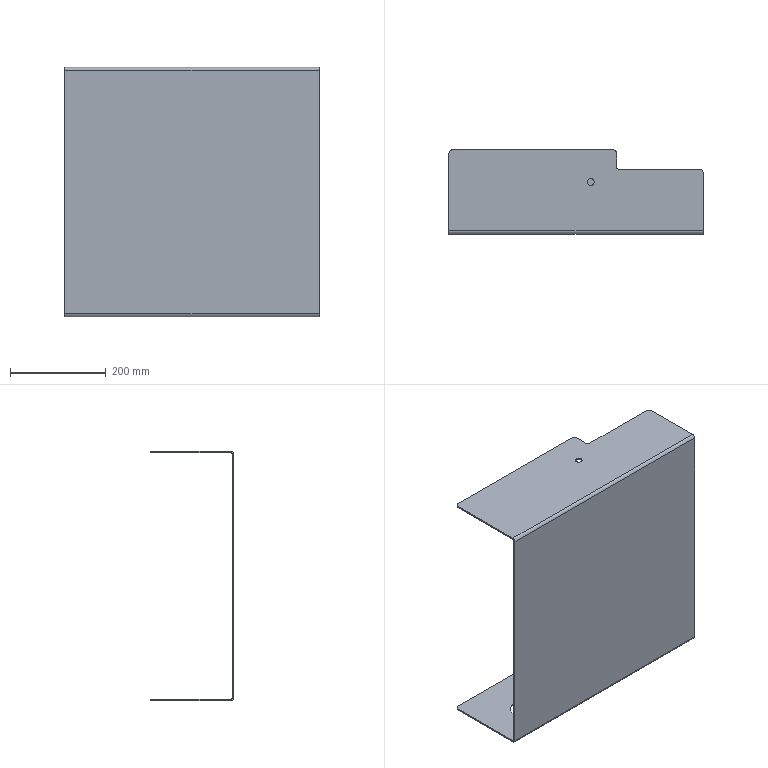Part | SolidWorks | features Fillet 2, ICE 2, FlatPattern 1, SMBaseFlange 1, SheetMetal 1 | 1 solid | 40 faces | box 530 x 175 x 520 mm | volume 1293540 mm3 | plane 22 | cylinder 18 | commonest cylinder face diameters 16 x6 6 x4 12 x2 14 x2 53 x2 100 x2
STEP:
#1=CARTESIAN_POINT('',(289.,-67.,-3.));
#2=VERTEX_POINT('',#1);
#3=CARTESIAN_POINT('',(303.,-67.,-3.));
#4=VERTEX_POINT('',#3);
#5=CARTESIAN_POINT('',(296.,-67.,-3.));
#6=DIRECTION('',(0.,0.,1.));
#7=DIRECTION('',(0.,1.,0.));
#8=AXIS2_PLACEMENT_3D('',#5,#6,#7);
#9=CIRCLE('',#8,7.);
#10=EDGE_CURVE('',#2,#4,#9,.T.);
#11=ORIENTED_EDGE('',*,*,#10,.F.);
#12=CARTESIAN_POINT('',(289.,-67.,0.));
#13=VERTEX_POINT('',#12);
#14=CARTESIAN_POINT('',(289.,-67.,-520.001));
#15=DIRECTION('',(0.,0.,1.));
#16=VECTOR('',#15,1000.);
#17=LINE('',#14,#16);
#18=EDGE_CURVE('',#2,#13,#17,.T.);
#19=ORIENTED_EDGE('',*,*,#18,.T.);
#20=CARTESIAN_POINT('',(303.,-67.,0.));
#21=VERTEX_POINT('',#20);
#22=CARTESIAN_POINT('',(296.,-67.,0.));
#23=DIRECTION('',(0.,0.,1.));
#24=DIRECTION('',(1.,0.,0.));
#25=AXIS2_PLACEMENT_3D('',#22,#23,#24);
#26=CIRCLE('',#25,7.);
#27=EDGE_CURVE('',#13,#21,#26,.T.);
#28=ORIENTED_EDGE('',*,*,#27,.T.);
#29=CARTESIAN_POINT('',(303.,-67.,-520.001));
#30=DIRECTION('',(0.,0.,1.));
#31=VECTOR('',#30,1000.);
#32=LINE('',#29,#31);
#33=EDGE_CURVE('',#4,#21,#32,.T.);
#34=ORIENTED_EDGE('',*,*,#33,.F.);
#35=EDGE_LOOP('',(#11,#19,#28,#34));
#36=FACE_OUTER_BOUND('',#35,.T.);
#37=CARTESIAN_POINT('',(296.,-67.,-520.001));
#38=DIRECTION('',(0.,0.,1.));
#39=DIRECTION('',(1.,0.,0.));
#40=AXIS2_PLACEMENT_3D('',#37,#38,#39);
#41=CYLINDRICAL_SURFACE('',#40,7.);
#42=ADVANCED_FACE('',(#36),#41,.F.);
#43=CARTESIAN_POINT('',(478.,-108.,-517.));
#44=VERTEX_POINT('',#43);
#45=CARTESIAN_POINT('',(378.,-108.,-517.));
#46=VERTEX_POINT('',#45);
#47=CARTESIAN_POINT('',(428.,-108.,-517.));
#48=DIRECTION('',(0.,0.,-1.));
#49=DIRECTION('',(1.,0.,0.));
#50=AXIS2_PLACEMENT_3D('',#47,#48,#49);
#51=CIRCLE('',#50,50.);
#52=EDGE_CURVE('',#44,#46,#51,.T.);
#53=ORIENTED_EDGE('',*,*,#52,.F.);
#54=CARTESIAN_POINT('',(478.,-108.,-520.));
#55=VERTEX_POINT('',#54);
#56=CARTESIAN_POINT('',(478.,-108.,0.001));
#57=DIRECTION('',(0.,0.,-1.));
#58=VECTOR('',#57,1000.);
#59=LINE('',#56,#58);
#60=EDGE_CURVE('',#44,#55,#59,.T.);
#61=ORIENTED_EDGE('',*,*,#60,.T.);
#62=CARTESIAN_POINT('',(378.,-108.,-520.));
#63=VERTEX_POINT('',#62);
#64=CARTESIAN_POINT('',(428.,-108.,-520.));
#65=DIRECTION('',(0.,0.,-1.));
#66=DIRECTION('',(-1.,0.,0.));
#67=AXIS2_PLACEMENT_3D('',#64,#65,#66);
#68=CIRCLE('',#67,50.);
#69=EDGE_CURVE('',#55,#63,#68,.T.);
#70=ORIENTED_EDGE('',*,*,#69,.T.);
#71=CARTESIAN_POINT('',(378.,-108.,0.001));
#72=DIRECTION('',(0.,0.,-1.));
#73=VECTOR('',#72,1000.);
#74=LINE('',#71,#73);
#75=EDGE_CURVE('',#46,#63,#74,.T.);
#76=ORIENTED_EDGE('',*,*,#75,.F.);
#77=EDGE_LOOP('',(#53,#61,#70,#76));
#78=FACE_OUTER_BOUND('',#77,.T.);
#79=CARTESIAN_POINT('',(428.,-108.,0.001));
#80=DIRECTION('',(0.,0.,-1.));
#81=DIRECTION('',(-1.,0.,0.));
#82=AXIS2_PLACEMENT_3D('',#79,#80,#81);
#83=CYLINDRICAL_SURFACE('',#82,50.);
#84=ADVANCED_FACE('',(#78),#83,.F.);
#85=CARTESIAN_POINT('',(122.5,-102.,-517.));
#86=VERTEX_POINT('',#85);
#87=CARTESIAN_POINT('',(69.5,-102.,-517.));
#88=VERTEX_POINT('',#87);
#89=CARTESIAN_POINT('',(96.,-102.,-517.));
#90=DIRECTION('',(0.,0.,-1.));
#91=DIRECTION('',(1.,0.,0.));
#92=AXIS2_PLACEMENT_3D('',#89,#90,#91);
#93=CIRCLE('',#92,26.5);
#94=EDGE_CURVE('',#86,#88,#93,.T.);
#95=ORIENTED_EDGE('',*,*,#94,.F.);
#96=CARTESIAN_POINT('',(122.5,-102.,-520.));
#97=VERTEX_POINT('',#96);
#98=CARTESIAN_POINT('',(122.5,-102.,0.001));
#99=DIRECTION('',(0.,0.,-1.));
#100=VECTOR('',#99,1000.);
#101=LINE('',#98,#100);
#102=EDGE_CURVE('',#86,#97,#101,.T.);
#103=ORIENTED_EDGE('',*,*,#102,.T.);
#104=CARTESIAN_POINT('',(69.5,-102.,-520.));
#105=VERTEX_POINT('',#104);
#106=CARTESIAN_POINT('',(96.,-102.,-520.));
#107=DIRECTION('',(0.,0.,-1.));
#108=DIRECTION('',(-1.,0.,0.));
#109=AXIS2_PLACEMENT_3D('',#106,#107,#108);
#110=CIRCLE('',#109,26.5);
#111=EDGE_CURVE('',#97,#105,#110,.T.);
#112=ORIENTED_EDGE('',*,*,#111,.T.);
#113=CARTESIAN_POINT('',(69.5,-102.,0.001));
#114=DIRECTION('',(0.,0.,-1.));
#115=VECTOR('',#114,1000.);
#116=LINE('',#113,#115);
#117=EDGE_CURVE('',#88,#105,#116,.T.);
#118=ORIENTED_EDGE('',*,*,#117,.F.);
#119=EDGE_LOOP('',(#95,#103,#112,#118));
#120=FACE_OUTER_BOUND('',#119,.T.);
#121=CARTESIAN_POINT('',(96.,-102.,0.001));
#122=DIRECTION('',(0.,0.,-1.));
#123=DIRECTION('',(-1.,0.,0.));
#124=AXIS2_PLACEMENT_3D('',#121,#122,#123);
#125=CYLINDRICAL_SURFACE('',#124,26.5);
#126=ADVANCED_FACE('',(#120),#125,.F.);
#127=CARTESIAN_POINT('',(530.,-169.,0.));
#128=VERTEX_POINT('',#127);
#129=CARTESIAN_POINT('',(530.,-169.,-3.));
#130=VERTEX_POINT('',#129);
#131=CARTESIAN_POINT('',(530.,-169.,0.));
#132=DIRECTION('',(0.,0.,-1.));
#133=VECTOR('',#132,1000.);
#134=LINE('',#131,#133);
#135=EDGE_CURVE('',#128,#130,#134,.T.);
#136=ORIENTED_EDGE('',*,*,#135,.F.);
#137=CARTESIAN_POINT('',(530.,-175.,-6.));
#138=VERTEX_POINT('',#137);
#139=CARTESIAN_POINT('',(530.,-169.,-6.));
#140=DIRECTION('',(1.,0.,0.));
#141=DIRECTION('',(0.,0.,1.));
#142=AXIS2_PLACEMENT_3D('',#139,#140,#141);
#143=CIRCLE('',#142,6.);
#144=EDGE_CURVE('',#128,#138,#143,.T.);
#145=ORIENTED_EDGE('',*,*,#144,.T.);
#146=CARTESIAN_POINT('',(530.,-172.,-6.));
#147=VERTEX_POINT('',#146);
#148=CARTESIAN_POINT('',(530.,-172.,-6.));
#149=DIRECTION('',(0.,-1.,0.));
#150=VECTOR('',#149,1000.);
#151=LINE('',#148,#150);
#152=EDGE_CURVE('',#147,#138,#151,.T.);
#153=ORIENTED_EDGE('',*,*,#152,.F.);
#154=CARTESIAN_POINT('',(530.,-169.,-6.));
#155=DIRECTION('',(1.,0.,0.));
#156=DIRECTION('',(0.,0.,-1.));
#157=AXIS2_PLACEMENT_3D('',#154,#155,#156);
#158=CIRCLE('',#157,3.);
#159=EDGE_CURVE('',#130,#147,#158,.T.);
#160=ORIENTED_EDGE('',*,*,#159,.F.);
#161=EDGE_LOOP('',(#136,#145,#153,#160));
#162=FACE_OUTER_BOUND('',#161,.T.);
#163=CARTESIAN_POINT('',(530.,-169.,0.));
#164=DIRECTION('',(1.,0.,0.));
#165=DIRECTION('',(0.,0.,-1.));
#166=AXIS2_PLACEMENT_3D('',#163,#164,#165);
#167=PLANE('',#166);
#168=ADVANCED_FACE('',(#162),#167,.T.);
#169=CARTESIAN_POINT('',(530.,-48.,-3.));
#170=VERTEX_POINT('',#169);
#171=CARTESIAN_POINT('',(530.,0.,-3.));
#172=DIRECTION('',(0.,-1.,0.));
#173=VECTOR('',#172,1000.);
#174=LINE('',#171,#173);
#175=EDGE_CURVE('',#170,#130,#174,.T.);
#176=ORIENTED_EDGE('',*,*,#175,.F.);
#177=CARTESIAN_POINT('',(530.,-48.,0.));
#178=VERTEX_POINT('',#177);
#179=CARTESIAN_POINT('',(530.,-48.,0.));
#180=DIRECTION('',(0.,0.,1.));
#181=VECTOR('',#180,1000.);
#182=LINE('',#179,#181);
#183=EDGE_CURVE('',#170,#178,#182,.T.);
#184=ORIENTED_EDGE('',*,*,#183,.T.);
#185=CARTESIAN_POINT('',(530.,0.,0.));
#186=DIRECTION('',(0.,-1.,0.));
#187=VECTOR('',#186,1000.);
#188=LINE('',#185,#187);
#189=EDGE_CURVE('',#178,#128,#188,.T.);
#190=ORIENTED_EDGE('',*,*,#189,.T.);
#191=ORIENTED_EDGE('',*,*,#135,.T.);
#192=EDGE_LOOP('',(#176,#184,#190,#191));
#193=FACE_OUTER_BOUND('',#192,.T.);
#194=CARTESIAN_POINT('',(530.,-172.,-6.));
#195=DIRECTION('',(1.,0.,0.));
#196=DIRECTION('',(0.,0.,-1.));
#197=AXIS2_PLACEMENT_3D('',#194,#195,#196);
#198=PLANE('',#197);
#199=ADVANCED_FACE('',(#193),#198,.T.);
#200=CARTESIAN_POINT('',(0.,-175.,-6.));
#201=VERTEX_POINT('',#200);
#202=CARTESIAN_POINT('',(0.,-172.,-6.));
#203=VERTEX_POINT('',#202);
#204=CARTESIAN_POINT('',(0.,-175.,-6.));
#205=DIRECTION('',(0.,1.,0.));
#206=VECTOR('',#205,1000.);
#207=LINE('',#204,#206);
#208=EDGE_CURVE('',#201,#203,#207,.T.);
#209=ORIENTED_EDGE('',*,*,#208,.F.);
#210=CARTESIAN_POINT('',(0.,-169.,0.));
#211=VERTEX_POINT('',#210);
#212=CARTESIAN_POINT('',(0.,-169.,-6.));
#213=DIRECTION('',(1.,0.,0.));
#214=DIRECTION('',(0.,0.,1.));
#215=AXIS2_PLACEMENT_3D('',#212,#213,#214);
#216=CIRCLE('',#215,6.);
#217=EDGE_CURVE('',#211,#201,#216,.T.);
#218=ORIENTED_EDGE('',*,*,#217,.F.);
#219=CARTESIAN_POINT('',(0.,-169.,-3.));
#220=VERTEX_POINT('',#219);
#221=CARTESIAN_POINT('',(0.,-169.,-3.));
#222=DIRECTION('',(0.,0.,1.));
#223=VECTOR('',#222,1000.);
#224=LINE('',#221,#223);
#225=EDGE_CURVE('',#220,#211,#224,.T.);
#226=ORIENTED_EDGE('',*,*,#225,.F.);
#227=CARTESIAN_POINT('',(0.,-169.,-6.));
#228=DIRECTION('',(1.,0.,0.));
#229=DIRECTION('',(0.,0.,-1.));
#230=AXIS2_PLACEMENT_3D('',#227,#228,#229);
#231=CIRCLE('',#230,3.);
#232=EDGE_CURVE('',#220,#203,#231,.T.);
#233=ORIENTED_EDGE('',*,*,#232,.T.);
#234=EDGE_LOOP('',(#209,#218,#226,#233));
#235=FACE_OUTER_BOUND('',#234,.T.);
#236=CARTESIAN_POINT('',(0.,-175.,-6.));
#237=DIRECTION('',(-1.,0.,0.));
#238=DIRECTION('',(0.,0.,1.));
#239=AXIS2_PLACEMENT_3D('',#236,#237,#238);
#240=PLANE('',#239);
#241=ADVANCED_FACE('',(#235),#240,.T.);
#242=CARTESIAN_POINT('',(0.,-175.,-514.));
#243=VERTEX_POINT('',#242);
#244=CARTESIAN_POINT('',(0.,-175.,0.));
#245=DIRECTION('',(0.,0.,-1.));
#246=VECTOR('',#245,1000.);
#247=LINE('',#244,#246);
#248=EDGE_CURVE('',#201,#243,#247,.T.);
#249=ORIENTED_EDGE('',*,*,#248,.F.);
#250=ORIENTED_EDGE('',*,*,#208,.T.);
#251=CARTESIAN_POINT('',(0.,-172.,-514.));
#252=VERTEX_POINT('',#251);
#253=CARTESIAN_POINT('',(0.,-172.,0.));
#254=DIRECTION('',(0.,0.,-1.));
#255=VECTOR('',#254,1000.);
#256=LINE('',#253,#255);
#257=EDGE_CURVE('',#203,#252,#256,.T.);
#258=ORIENTED_EDGE('',*,*,#257,.T.);
#259=CARTESIAN_POINT('',(0.,-172.,-514.));
#260=DIRECTION('',(0.,-1.,0.));
#261=VECTOR('',#260,1000.);
#262=LINE('',#259,#261);
#263=EDGE_CURVE('',#252,#243,#262,.T.);
#264=ORIENTED_EDGE('',*,*,#263,.T.);
#265=EDGE_LOOP('',(#249,#250,#258,#264));
#266=FACE_OUTER_BOUND('',#265,.T.);
#267=CARTESIAN_POINT('',(0.,-169.,-3.));
#268=DIRECTION('',(-1.,0.,0.));
#269=DIRECTION('',(0.,0.,1.));
#270=AXIS2_PLACEMENT_3D('',#267,#268,#269);
#271=PLANE('',#270);
#272=ADVANCED_FACE('',(#266),#271,.T.);
#273=CARTESIAN_POINT('',(530.,-175.,-514.));
#274=VERTEX_POINT('',#273);
#275=CARTESIAN_POINT('',(530.,-172.,-514.));
#276=VERTEX_POINT('',#275);
#277=CARTESIAN_POINT('',(530.,-175.,-514.));
#278=DIRECTION('',(0.,1.,0.));
#279=VECTOR('',#278,1000.);
#280=LINE('',#277,#279);
#281=EDGE_CURVE('',#274,#276,#280,.T.);
#282=ORIENTED_EDGE('',*,*,#281,.F.);
#283=CARTESIAN_POINT('',(530.,-169.,-520.));
#284=VERTEX_POINT('',#283);
#285=CARTESIAN_POINT('',(530.,-169.,-514.));
#286=DIRECTION('',(1.,0.,0.));
#287=DIRECTION('',(0.,0.,1.));
#288=AXIS2_PLACEMENT_3D('',#285,#286,#287);
#289=CIRCLE('',#288,6.);
#290=EDGE_CURVE('',#274,#284,#289,.T.);
#291=ORIENTED_EDGE('',*,*,#290,.T.);
#292=CARTESIAN_POINT('',(530.,-169.,-517.));
#293=VERTEX_POINT('',#292);
#294=CARTESIAN_POINT('',(530.,-169.,-517.));
#295=DIRECTION('',(0.,0.,-1.));
#296=VECTOR('',#295,1000.);
#297=LINE('',#294,#296);
#298=EDGE_CURVE('',#293,#284,#297,.T.);
#299=ORIENTED_EDGE('',*,*,#298,.F.);
#300=CARTESIAN_POINT('',(530.,-169.,-514.));
#301=DIRECTION('',(1.,0.,0.));
#302=DIRECTION('',(0.,0.,-1.));
#303=AXIS2_PLACEMENT_3D('',#300,#301,#302);
#304=CIRCLE('',#303,3.);
#305=EDGE_CURVE('',#276,#293,#304,.T.);
#306=ORIENTED_EDGE('',*,*,#305,.F.);
#307=EDGE_LOOP('',(#282,#291,#299,#306));
#308=FACE_OUTER_BOUND('',#307,.T.);
#309=CARTESIAN_POINT('',(530.,-175.,-514.));
#310=DIRECTION('',(1.,0.,0.));
#311=DIRECTION('',(0.,0.,-1.));
#312=AXIS2_PLACEMENT_3D('',#309,#310,#311);
#313=PLANE('',#312);
#314=ADVANCED_FACE('',(#308),#313,.T.);
#315=CARTESIAN_POINT('',(530.,-175.,0.));
#316=DIRECTION('',(0.,0.,-1.));
#317=VECTOR('',#316,1000.);
#318=LINE('',#315,#317);
#319=EDGE_CURVE('',#138,#274,#318,.T.);
#320=ORIENTED_EDGE('',*,*,#319,.T.);
#321=ORIENTED_EDGE('',*,*,#281,.T.);
#322=CARTESIAN_POINT('',(530.,-172.,0.));
#323=DIRECTION('',(0.,0.,-1.));
#324=VECTOR('',#323,1000.);
#325=LINE('',#322,#324);
#326=EDGE_CURVE('',#147,#276,#325,.T.);
#327=ORIENTED_EDGE('',*,*,#326,.F.);
#328=ORIENTED_EDGE('',*,*,#152,.T.);
#329=EDGE_LOOP('',(#320,#321,#327,#328));
#330=FACE_OUTER_BOUND('',#329,.T.);
#331=CARTESIAN_POINT('',(530.,-169.,-517.));
#332=DIRECTION('',(1.,0.,0.));
#333=DIRECTION('',(0.,0.,-1.));
#334=AXIS2_PLACEMENT_3D('',#331,#332,#333);
#335=PLANE('',#334);
#336=ADVANCED_FACE('',(#330),#335,.T.);
#337=CARTESIAN_POINT('',(0.,-169.,-520.));
#338=VERTEX_POINT('',#337);
#339=CARTESIAN_POINT('',(0.,-169.,-517.));
#340=VERTEX_POINT('',#339);
#341=CARTESIAN_POINT('',(0.,-169.,-520.));
#342=DIRECTION('',(0.,0.,1.));
#343=VECTOR('',#342,1000.);
#344=LINE('',#341,#343);
#345=EDGE_CURVE('',#338,#340,#344,.T.);
#346=ORIENTED_EDGE('',*,*,#345,.F.);
#347=CARTESIAN_POINT('',(0.,-169.,-514.));
#348=DIRECTION('',(1.,0.,0.));
#349=DIRECTION('',(0.,0.,1.));
#350=AXIS2_PLACEMENT_3D('',#347,#348,#349);
#351=CIRCLE('',#350,6.);
#352=EDGE_CURVE('',#243,#338,#351,.T.);
#353=ORIENTED_EDGE('',*,*,#352,.F.);
#354=ORIENTED_EDGE('',*,*,#263,.F.);
#355=CARTESIAN_POINT('',(0.,-169.,-514.));
#356=DIRECTION('',(1.,0.,0.));
#357=DIRECTION('',(0.,0.,-1.));
#358=AXIS2_PLACEMENT_3D('',#355,#356,#357);
#359=CIRCLE('',#358,3.);
#360=EDGE_CURVE('',#252,#340,#359,.T.);
#361=ORIENTED_EDGE('',*,*,#360,.T.);
#362=EDGE_LOOP('',(#346,#353,#354,#361));
#363=FACE_OUTER_BOUND('',#362,.T.);
#364=CARTESIAN_POINT('',(0.,-169.,-520.));
#365=DIRECTION('',(-1.,0.,0.));
#366=DIRECTION('',(0.,0.,1.));
#367=AXIS2_PLACEMENT_3D('',#364,#365,#366);
#368=PLANE('',#367);
#369=ADVANCED_FACE('',(#363),#368,.T.);
#370=CARTESIAN_POINT('',(0.,-8.,-517.));
#371=VERTEX_POINT('',#370);
#372=CARTESIAN_POINT('',(0.,-175.,-517.));
#373=DIRECTION('',(0.,1.,0.));
#374=VECTOR('',#373,1000.);
#375=LINE('',#372,#374);
#376=EDGE_CURVE('',#340,#371,#375,.T.);
#377=ORIENTED_EDGE('',*,*,#376,.T.);
#378=CARTESIAN_POINT('',(0.,-8.,-520.));
#379=VERTEX_POINT('',#378);
#380=CARTESIAN_POINT('',(0.,-8.,-514.));
#381=DIRECTION('',(0.,0.,-1.));
#382=VECTOR('',#381,1000.);
#383=LINE('',#380,#382);
#384=EDGE_CURVE('',#371,#379,#383,.T.);
#385=ORIENTED_EDGE('',*,*,#384,.T.);
#386=CARTESIAN_POINT('',(0.,-175.,-520.));
#387=DIRECTION('',(0.,1.,0.));
#388=VECTOR('',#387,1000.);
#389=LINE('',#386,#388);
#390=EDGE_CURVE('',#338,#379,#389,.T.);
#391=ORIENTED_EDGE('',*,*,#390,.F.);
#392=ORIENTED_EDGE('',*,*,#345,.T.);
#393=EDGE_LOOP('',(#377,#385,#391,#392));
#394=FACE_OUTER_BOUND('',#393,.T.);
#395=CARTESIAN_POINT('',(0.,-172.,-514.));
#396=DIRECTION('',(-1.,0.,0.));
#397=DIRECTION('',(0.,0.,1.));
#398=AXIS2_PLACEMENT_3D('',#395,#396,#397);
#399=PLANE('',#398);
#400=ADVANCED_FACE('',(#394),#399,.T.);
#401=CARTESIAN_POINT('',(428.,-108.,-520.));
#402=DIRECTION('',(0.,0.,-1.));
#403=DIRECTION('',(-1.,0.,0.));
#404=AXIS2_PLACEMENT_3D('',#401,#402,#403);
#405=CIRCLE('',#404,50.);
#406=EDGE_CURVE('',#63,#55,#405,.T.);
#407=ORIENTED_EDGE('',*,*,#406,.F.);
#408=ORIENTED_EDGE('',*,*,#69,.F.);
#409=EDGE_LOOP('',(#407,#408));
#410=FACE_BOUND('',#409,.T.);
#411=CARTESIAN_POINT('',(96.,-102.,-520.));
#412=DIRECTION('',(0.,0.,-1.));
#413=DIRECTION('',(-1.,0.,0.));
#414=AXIS2_PLACEMENT_3D('',#411,#412,#413);
#415=CIRCLE('',#414,26.5);
#416=EDGE_CURVE('',#105,#97,#415,.T.);
#417=ORIENTED_EDGE('',*,*,#416,.F.);
#418=ORIENTED_EDGE('',*,*,#111,.F.);
#419=EDGE_LOOP('',(#417,#418));
#420=FACE_BOUND('',#419,.T.);
#421=ORIENTED_EDGE('',*,*,#390,.T.);
#422=CARTESIAN_POINT('',(8.,0.,-520.));
#423=VERTEX_POINT('',#422);
#424=CARTESIAN_POINT('',(8.,-8.,-520.));
#425=DIRECTION('',(0.,0.,-1.));
#426=DIRECTION('',(1.,0.,0.));
#427=AXIS2_PLACEMENT_3D('',#424,#425,#426);
#428=CIRCLE('',#427,8.);
#429=EDGE_CURVE('',#379,#423,#428,.T.);
#430=ORIENTED_EDGE('',*,*,#429,.T.);
#431=CARTESIAN_POINT('',(342.,0.,-520.));
#432=VERTEX_POINT('',#431);
#433=CARTESIAN_POINT('',(530.,0.,-520.));
#434=DIRECTION('',(-1.,0.,0.));
#435=VECTOR('',#434,1000.);
#436=LINE('',#433,#435);
#437=EDGE_CURVE('',#432,#423,#436,.T.);
#438=ORIENTED_EDGE('',*,*,#437,.F.);
#439=CARTESIAN_POINT('',(350.,-8.,-520.));
#440=VERTEX_POINT('',#439);
#441=CARTESIAN_POINT('',(342.,-8.,-520.));
#442=DIRECTION('',(0.,0.,-1.));
#443=DIRECTION('',(1.,0.,0.));
#444=AXIS2_PLACEMENT_3D('',#441,#442,#443);
#445=CIRCLE('',#444,8.);
#446=EDGE_CURVE('',#432,#440,#445,.T.);
#447=ORIENTED_EDGE('',*,*,#446,.T.);
#448=CARTESIAN_POINT('',(350.,-37.,-520.));
#449=VERTEX_POINT('',#448);
#450=CARTESIAN_POINT('',(350.,0.,-520.));
#451=DIRECTION('',(0.,1.,0.));
#452=VECTOR('',#451,1000.);
#453=LINE('',#450,#452);
#454=EDGE_CURVE('',#449,#440,#453,.T.);
#455=ORIENTED_EDGE('',*,*,#454,.F.);
#456=CARTESIAN_POINT('',(353.,-40.,-520.));
#457=VERTEX_POINT('',#456);
#458=CARTESIAN_POINT('',(353.,-37.,-520.));
#459=DIRECTION('',(0.,0.,1.));
#460=DIRECTION('',(1.,0.,0.));
#461=AXIS2_PLACEMENT_3D('',#458,#459,#460);
#462=CIRCLE('',#461,3.);
#463=EDGE_CURVE('',#449,#457,#462,.T.);
#464=ORIENTED_EDGE('',*,*,#463,.T.);
#465=CARTESIAN_POINT('',(522.,-40.,-520.));
#466=VERTEX_POINT('',#465);
#467=CARTESIAN_POINT('',(530.,-40.,-520.));
#468=DIRECTION('',(-1.,0.,0.));
#469=VECTOR('',#468,1000.);
#470=LINE('',#467,#469);
#471=EDGE_CURVE('',#466,#457,#470,.T.);
#472=ORIENTED_EDGE('',*,*,#471,.F.);
#473=CARTESIAN_POINT('',(530.,-48.,-520.));
#474=VERTEX_POINT('',#473);
#475=CARTESIAN_POINT('',(522.,-48.,-520.));
#476=DIRECTION('',(0.,0.,-1.));
#477=DIRECTION('',(1.,0.,0.));
#478=AXIS2_PLACEMENT_3D('',#475,#476,#477);
#479=CIRCLE('',#478,8.);
#480=EDGE_CURVE('',#466,#474,#479,.T.);
#481=ORIENTED_EDGE('',*,*,#480,.T.);
#482=CARTESIAN_POINT('',(530.,-175.,-520.));
#483=DIRECTION('',(0.,1.,0.));
#484=VECTOR('',#483,1000.);
#485=LINE('',#482,#484);
#486=EDGE_CURVE('',#284,#474,#485,.T.);
#487=ORIENTED_EDGE('',*,*,#486,.F.);
#488=CARTESIAN_POINT('',(530.,-169.,-520.));
#489=DIRECTION('',(-1.,0.,0.));
#490=VECTOR('',#489,1000.);
#491=LINE('',#488,#490);
#492=EDGE_CURVE('',#284,#338,#491,.T.);
#493=ORIENTED_EDGE('',*,*,#492,.T.);
#494=EDGE_LOOP('',(#421,#430,#438,#447,#455,#464,#472,#481,#487,#493));
#495=FACE_OUTER_BOUND('',#494,.T.);
#496=CARTESIAN_POINT('',(530.,-175.,-520.));
#497=DIRECTION('',(0.,0.,1.));
#498=DIRECTION('',(1.,0.,0.));
#499=AXIS2_PLACEMENT_3D('',#496,#497,#498);
#500=PLANE('',#499);
#501=ADVANCED_FACE('',(#410,#420,#495),#500,.F.);
#502=ORIENTED_EDGE('',*,*,#437,.T.);
#503=CARTESIAN_POINT('',(8.,0.,-517.));
#504=VERTEX_POINT('',#503);
#505=CARTESIAN_POINT('',(8.,0.,-517.));
#506=DIRECTION('',(0.,0.,1.));
#507=VECTOR('',#506,1000.);
#508=LINE('',#505,#507);
#509=EDGE_CURVE('',#423,#504,#508,.T.);
#510=ORIENTED_EDGE('',*,*,#509,.T.);
#511=CARTESIAN_POINT('',(342.,0.,-517.));
#512=VERTEX_POINT('',#511);
#513=CARTESIAN_POINT('',(530.,0.,-517.));
#514=DIRECTION('',(-1.,0.,0.));
#515=VECTOR('',#514,1000.);
#516=LINE('',#513,#515);
#517=EDGE_CURVE('',#512,#504,#516,.T.);
#518=ORIENTED_EDGE('',*,*,#517,.F.);
#519=CARTESIAN_POINT('',(342.,0.,-520.));
#520=DIRECTION('',(0.,0.,-1.));
#521=VECTOR('',#520,1000.);
#522=LINE('',#519,#521);
#523=EDGE_CURVE('',#512,#432,#522,.T.);
#524=ORIENTED_EDGE('',*,*,#523,.T.);
#525=EDGE_LOOP('',(#502,#510,#518,#524));
#526=FACE_OUTER_BOUND('',#525,.T.);
#527=CARTESIAN_POINT('',(530.,0.,-517.));
#528=DIRECTION('',(0.,1.,0.));
#529=DIRECTION('',(0.,0.,1.));
#530=AXIS2_PLACEMENT_3D('',#527,#528,#529);
#531=PLANE('',#530);
#532=ADVANCED_FACE('',(#526),#531,.T.);
#533=ORIENTED_EDGE('',*,*,#517,.T.);
#534=CARTESIAN_POINT('',(8.,-8.,-517.));
#535=DIRECTION('',(0.,0.,1.));
#536=DIRECTION('',(1.,0.,0.));
#537=AXIS2_PLACEMENT_3D('',#534,#535,#536);
#538=CIRCLE('',#537,8.);
#539=EDGE_CURVE('',#504,#371,#538,.T.);
#540=ORIENTED_EDGE('',*,*,#539,.T.);
#541=ORIENTED_EDGE('',*,*,#376,.F.);
#542=CARTESIAN_POINT('',(530.,-169.,-517.));
#543=DIRECTION('',(-1.,0.,0.));
#544=VECTOR('',#543,1000.);
#545=LINE('',#542,#544);
#546=EDGE_CURVE('',#293,#340,#545,.T.);
#547=ORIENTED_EDGE('',*,*,#546,.F.);
#548=CARTESIAN_POINT('',(530.,-48.,-517.));
#549=VERTEX_POINT('',#548);
#550=CARTESIAN_POINT('',(530.,-175.,-517.));
#551=DIRECTION('',(0.,1.,0.));
#552=VECTOR('',#551,1000.);
#553=LINE('',#550,#552);
#554=EDGE_CURVE('',#293,#549,#553,.T.);
#555=ORIENTED_EDGE('',*,*,#554,.T.);
#556=CARTESIAN_POINT('',(522.,-40.,-517.));
#557=VERTEX_POINT('',#556);
#558=CARTESIAN_POINT('',(522.,-48.,-517.));
#559=DIRECTION('',(0.,0.,1.));
#560=DIRECTION('',(1.,0.,0.));
#561=AXIS2_PLACEMENT_3D('',#558,#559,#560);
#562=CIRCLE('',#561,8.);
#563=EDGE_CURVE('',#549,#557,#562,.T.);
#564=ORIENTED_EDGE('',*,*,#563,.T.);
#565=CARTESIAN_POINT('',(353.,-40.,-517.));
#566=VERTEX_POINT('',#565);
#567=CARTESIAN_POINT('',(530.,-40.,-517.));
#568=DIRECTION('',(-1.,0.,0.));
#569=VECTOR('',#568,1000.);
#570=LINE('',#567,#569);
#571=EDGE_CURVE('',#557,#566,#570,.T.);
#572=ORIENTED_EDGE('',*,*,#571,.T.);
#573=CARTESIAN_POINT('',(350.,-37.,-517.));
#574=VERTEX_POINT('',#573);
#575=CARTESIAN_POINT('',(353.,-37.,-517.));
#576=DIRECTION('',(0.,0.,-1.));
#577=DIRECTION('',(1.,0.,0.));
#578=AXIS2_PLACEMENT_3D('',#575,#576,#577);
#579=CIRCLE('',#578,3.);
#580=EDGE_CURVE('',#566,#574,#579,.T.);
#581=ORIENTED_EDGE('',*,*,#580,.T.);
#582=CARTESIAN_POINT('',(350.,-8.,-517.));
#583=VERTEX_POINT('',#582);
#584=CARTESIAN_POINT('',(350.,0.,-517.));
#585=DIRECTION('',(0.,1.,0.));
#586=VECTOR('',#585,1000.);
#587=LINE('',#584,#586);
#588=EDGE_CURVE('',#574,#583,#587,.T.);
#589=ORIENTED_EDGE('',*,*,#588,.T.);
#590=CARTESIAN_POINT('',(342.,-8.,-517.));
#591=DIRECTION('',(0.,0.,1.));
#592=DIRECTION('',(1.,0.,0.));
#593=AXIS2_PLACEMENT_3D('',#590,#591,#592);
#594=CIRCLE('',#593,8.);
#595=EDGE_CURVE('',#583,#512,#594,.T.);
#596=ORIENTED_EDGE('',*,*,#595,.T.);
#597=EDGE_LOOP('',(#533,#540,#541,#547,#555,#564,#572,#581,#589,#596));
#598=FACE_OUTER_BOUND('',#597,.T.);
#599=CARTESIAN_POINT('',(428.,-108.,-517.));
#600=DIRECTION('',(0.,0.,-1.));
#601=DIRECTION('',(1.,0.,0.));
#602=AXIS2_PLACEMENT_3D('',#599,#600,#601);
#603=CIRCLE('',#602,50.);
#604=EDGE_CURVE('',#46,#44,#603,.T.);
#605=ORIENTED_EDGE('',*,*,#604,.T.);
#606=ORIENTED_EDGE('',*,*,#52,.T.);
#607=EDGE_LOOP('',(#605,#606));
#608=FACE_BOUND('',#607,.T.);
#609=CARTESIAN_POINT('',(96.,-102.,-517.));
#610=DIRECTION('',(0.,0.,-1.));
#611=DIRECTION('',(1.,0.,0.));
#612=AXIS2_PLACEMENT_3D('',#609,#610,#611);
#613=CIRCLE('',#612,26.5);
#614=EDGE_CURVE('',#88,#86,#613,.T.);
#615=ORIENTED_EDGE('',*,*,#614,.T.);
#616=ORIENTED_EDGE('',*,*,#94,.T.);
#617=EDGE_LOOP('',(#615,#616));
#618=FACE_BOUND('',#617,.T.);
#619=CARTESIAN_POINT('',(530.,-175.,-517.));
#620=DIRECTION('',(0.,0.,1.));
#621=DIRECTION('',(1.,0.,0.));
#622=AXIS2_PLACEMENT_3D('',#619,#620,#621);
#623=PLANE('',#622);
#624=ADVANCED_FACE('',(#598,#608,#618),#623,.T.);
#625=ORIENTED_EDGE('',*,*,#360,.F.);
#626=CARTESIAN_POINT('',(530.,-172.,-514.));
#627=DIRECTION('',(-1.,0.,0.));
#628=VECTOR('',#627,1000.);
#629=LINE('',#626,#628);
#630=EDGE_CURVE('',#276,#252,#629,.T.);
#631=ORIENTED_EDGE('',*,*,#630,.F.);
#632=ORIENTED_EDGE('',*,*,#305,.T.);
#633=ORIENTED_EDGE('',*,*,#546,.T.);
#634=EDGE_LOOP('',(#625,#631,#632,#633));
#635=FACE_OUTER_BOUND('',#634,.T.);
#636=CARTESIAN_POINT('',(530.,-169.,-514.));
#637=DIRECTION('',(-1.,0.,0.));
#638=DIRECTION('',(0.,0.,1.));
#639=AXIS2_PLACEMENT_3D('',#636,#637,#638);
#640=CYLINDRICAL_SURFACE('',#639,3.);
#641=ADVANCED_FACE('',(#635),#640,.F.);
#642=ORIENTED_EDGE('',*,*,#257,.F.);
#643=CARTESIAN_POINT('',(530.,-172.,-6.));
#644=DIRECTION('',(-1.,0.,0.));
#645=VECTOR('',#644,1000.);
#646=LINE('',#643,#645);
#647=EDGE_CURVE('',#147,#203,#646,.T.);
#648=ORIENTED_EDGE('',*,*,#647,.F.);
#649=ORIENTED_EDGE('',*,*,#326,.T.);
#650=ORIENTED_EDGE('',*,*,#630,.T.);
#651=EDGE_LOOP('',(#642,#648,#649,#650));
#652=FACE_OUTER_BOUND('',#651,.T.);
#653=CARTESIAN_POINT('',(530.,-172.,0.));
#654=DIRECTION('',(0.,1.,0.));
#655=DIRECTION('',(0.,0.,1.));
#656=AXIS2_PLACEMENT_3D('',#653,#654,#655);
#657=PLANE('',#656);
#658=ADVANCED_FACE('',(#652),#657,.T.);
#659=ORIENTED_EDGE('',*,*,#232,.F.);
#660=CARTESIAN_POINT('',(530.,-169.,-3.));
#661=DIRECTION('',(-1.,0.,0.));
#662=VECTOR('',#661,1000.);
#663=LINE('',#660,#662);
#664=EDGE_CURVE('',#130,#220,#663,.T.);
#665=ORIENTED_EDGE('',*,*,#664,.F.);
#666=ORIENTED_EDGE('',*,*,#159,.T.);
#667=ORIENTED_EDGE('',*,*,#647,.T.);
#668=EDGE_LOOP('',(#659,#665,#666,#667));
#669=FACE_OUTER_BOUND('',#668,.T.);
#670=CARTESIAN_POINT('',(530.,-169.,-6.));
#671=DIRECTION('',(-1.,0.,0.));
#672=DIRECTION('',(0.,0.,1.));
#673=AXIS2_PLACEMENT_3D('',#670,#671,#672);
#674=CYLINDRICAL_SURFACE('',#673,3.);
#675=ADVANCED_FACE('',(#669),#674,.F.);
#676=CARTESIAN_POINT('',(350.,-8.,-3.));
#677=VERTEX_POINT('',#676);
#678=CARTESIAN_POINT('',(350.,-37.,-3.));
#679=VERTEX_POINT('',#678);
#680=CARTESIAN_POINT('',(350.,0.,-3.));
#681=DIRECTION('',(0.,-1.,0.));
#682=VECTOR('',#681,1000.);
#683=LINE('',#680,#682);
#684=EDGE_CURVE('',#677,#679,#683,.T.);
#685=ORIENTED_EDGE('',*,*,#684,.T.);
#686=CARTESIAN_POINT('',(353.,-40.,-3.));
#687=VERTEX_POINT('',#686);
#688=CARTESIAN_POINT('',(353.,-37.,-3.));
#689=DIRECTION('',(0.,0.,1.));
#690=DIRECTION('',(0.,1.,0.));
#691=AXIS2_PLACEMENT_3D('',#688,#689,#690);
#692=CIRCLE('',#691,3.);
#693=EDGE_CURVE('',#679,#687,#692,.T.);
#694=ORIENTED_EDGE('',*,*,#693,.T.);
#695=CARTESIAN_POINT('',(522.,-40.,-3.));
#696=VERTEX_POINT('',#695);
#697=CARTESIAN_POINT('',(530.,-40.,-3.));
#698=DIRECTION('',(1.,0.,0.));
#699=VECTOR('',#698,1000.);
#700=LINE('',#697,#699);
#701=EDGE_CURVE('',#687,#696,#700,.T.);
#702=ORIENTED_EDGE('',*,*,#701,.T.);
#703=CARTESIAN_POINT('',(522.,-48.,-3.));
#704=DIRECTION('',(0.,0.,-1.));
#705=DIRECTION('',(0.,1.,0.));
#706=AXIS2_PLACEMENT_3D('',#703,#704,#705);
#707=CIRCLE('',#706,8.);
#708=EDGE_CURVE('',#696,#170,#707,.T.);
#709=ORIENTED_EDGE('',*,*,#708,.T.);
#710=ORIENTED_EDGE('',*,*,#175,.T.);
#711=ORIENTED_EDGE('',*,*,#664,.T.);
#712=CARTESIAN_POINT('',(0.,-8.,-3.));
#713=VERTEX_POINT('',#712);
#714=CARTESIAN_POINT('',(0.,0.,-3.));
#715=DIRECTION('',(0.,-1.,0.));
#716=VECTOR('',#715,1000.);
#717=LINE('',#714,#716);
#718=EDGE_CURVE('',#713,#220,#717,.T.);
#719=ORIENTED_EDGE('',*,*,#718,.F.);
#720=CARTESIAN_POINT('',(8.,0.,-3.));
#721=VERTEX_POINT('',#720);
#722=CARTESIAN_POINT('',(8.,-8.,-3.));
#723=DIRECTION('',(0.,0.,-1.));
#724=DIRECTION('',(0.,1.,0.));
#725=AXIS2_PLACEMENT_3D('',#722,#723,#724);
#726=CIRCLE('',#725,8.);
#727=EDGE_CURVE('',#713,#721,#726,.T.);
#728=ORIENTED_EDGE('',*,*,#727,.T.);
#729=CARTESIAN_POINT('',(342.,0.,-3.));
#730=VERTEX_POINT('',#729);
#731=CARTESIAN_POINT('',(530.,0.,-3.));
#732=DIRECTION('',(-1.,0.,0.));
#733=VECTOR('',#732,1000.);
#734=LINE('',#731,#733);
#735=EDGE_CURVE('',#730,#721,#734,.T.);
#736=ORIENTED_EDGE('',*,*,#735,.F.);
#737=CARTESIAN_POINT('',(342.,-8.,-3.));
#738=DIRECTION('',(0.,0.,-1.));
#739=DIRECTION('',(0.,1.,0.));
#740=AXIS2_PLACEMENT_3D('',#737,#738,#739);
#741=CIRCLE('',#740,8.);
#742=EDGE_CURVE('',#730,#677,#741,.T.);
#743=ORIENTED_EDGE('',*,*,#742,.T.);
#744=EDGE_LOOP('',(#685,#694,#702,#709,#710,#711,#719,#728,#736,#743));
#745=FACE_OUTER_BOUND('',#744,.T.);
#746=CARTESIAN_POINT('',(296.,-67.,-3.));
#747=DIRECTION('',(0.,0.,1.));
#748=DIRECTION('',(0.,1.,0.));
#749=AXIS2_PLACEMENT_3D('',#746,#747,#748);
#750=CIRCLE('',#749,7.);
#751=EDGE_CURVE('',#4,#2,#750,.T.);
#752=ORIENTED_EDGE('',*,*,#751,.T.);
#753=ORIENTED_EDGE('',*,*,#10,.T.);
#754=EDGE_LOOP('',(#752,#753));
#755=FACE_BOUND('',#754,.T.);
#756=CARTESIAN_POINT('',(530.,0.,-3.));
#757=DIRECTION('',(0.,0.,-1.));
#758=DIRECTION('',(0.,1.,0.));
#759=AXIS2_PLACEMENT_3D('',#756,#757,#758);
#760=PLANE('',#759);
#761=ADVANCED_FACE('',(#745,#755),#760,.T.);
#762=CARTESIAN_POINT('',(342.,0.,0.));
#763=VERTEX_POINT('',#762);
#764=CARTESIAN_POINT('',(8.,0.,0.));
#765=VERTEX_POINT('',#764);
#766=CARTESIAN_POINT('',(530.,0.,0.));
#767=DIRECTION('',(-1.,0.,0.));
#768=VECTOR('',#767,1000.);
#769=LINE('',#766,#768);
#770=EDGE_CURVE('',#763,#765,#769,.T.);
#771=ORIENTED_EDGE('',*,*,#770,.F.);
#772=CARTESIAN_POINT('',(342.,0.,-3.));
#773=DIRECTION('',(0.,0.,-1.));
#774=VECTOR('',#773,1000.);
#775=LINE('',#772,#774);
#776=EDGE_CURVE('',#763,#730,#775,.T.);
#777=ORIENTED_EDGE('',*,*,#776,.T.);
#778=ORIENTED_EDGE('',*,*,#735,.T.);
#779=CARTESIAN_POINT('',(8.,0.,0.));
#780=DIRECTION('',(0.,0.,1.));
#781=VECTOR('',#780,1000.);
#782=LINE('',#779,#781);
#783=EDGE_CURVE('',#721,#765,#782,.T.);
#784=ORIENTED_EDGE('',*,*,#783,.T.);
#785=EDGE_LOOP('',(#771,#777,#778,#784));
#786=FACE_OUTER_BOUND('',#785,.T.);
#787=CARTESIAN_POINT('',(530.,0.,0.));
#788=DIRECTION('',(0.,1.,0.));
#789=DIRECTION('',(0.,0.,1.));
#790=AXIS2_PLACEMENT_3D('',#787,#788,#789);
#791=PLANE('',#790);
#792=ADVANCED_FACE('',(#786),#791,.T.);
#793=CARTESIAN_POINT('',(296.,-67.,0.));
#794=DIRECTION('',(0.,0.,1.));
#795=DIRECTION('',(1.,0.,0.));
#796=AXIS2_PLACEMENT_3D('',#793,#794,#795);
#797=CIRCLE('',#796,7.);
#798=EDGE_CURVE('',#21,#13,#797,.T.);
#799=ORIENTED_EDGE('',*,*,#798,.F.);
#800=ORIENTED_EDGE('',*,*,#27,.F.);
#801=EDGE_LOOP('',(#799,#800));
#802=FACE_BOUND('',#801,.T.);
#803=ORIENTED_EDGE('',*,*,#189,.F.);
#804=CARTESIAN_POINT('',(522.,-40.,0.));
#805=VERTEX_POINT('',#804);
#806=CARTESIAN_POINT('',(522.,-48.,0.));
#807=DIRECTION('',(0.,0.,1.));
#808=DIRECTION('',(0.,1.,0.));
#809=AXIS2_PLACEMENT_3D('',#806,#807,#808);
#810=CIRCLE('',#809,8.);
#811=EDGE_CURVE('',#178,#805,#810,.T.);
#812=ORIENTED_EDGE('',*,*,#811,.T.);
#813=CARTESIAN_POINT('',(353.,-40.,0.));
#814=VERTEX_POINT('',#813);
#815=CARTESIAN_POINT('',(530.,-40.,0.));
#816=DIRECTION('',(1.,0.,0.));
#817=VECTOR('',#816,1000.);
#818=LINE('',#815,#817);
#819=EDGE_CURVE('',#814,#805,#818,.T.);
#820=ORIENTED_EDGE('',*,*,#819,.F.);
#821=CARTESIAN_POINT('',(350.,-37.,0.));
#822=VERTEX_POINT('',#821);
#823=CARTESIAN_POINT('',(353.,-37.,0.));
#824=DIRECTION('',(0.,0.,-1.));
#825=DIRECTION('',(0.,1.,0.));
#826=AXIS2_PLACEMENT_3D('',#823,#824,#825);
#827=CIRCLE('',#826,3.);
#828=EDGE_CURVE('',#814,#822,#827,.T.);
#829=ORIENTED_EDGE('',*,*,#828,.T.);
#830=CARTESIAN_POINT('',(350.,-8.,0.));
#831=VERTEX_POINT('',#830);
#832=CARTESIAN_POINT('',(350.,0.,0.));
#833=DIRECTION('',(0.,-1.,0.));
#834=VECTOR('',#833,1000.);
#835=LINE('',#832,#834);
#836=EDGE_CURVE('',#831,#822,#835,.T.);
#837=ORIENTED_EDGE('',*,*,#836,.F.);
#838=CARTESIAN_POINT('',(342.,-8.,0.));
#839=DIRECTION('',(0.,0.,1.));
#840=DIRECTION('',(0.,1.,0.));
#841=AXIS2_PLACEMENT_3D('',#838,#839,#840);
#842=CIRCLE('',#841,8.);
#843=EDGE_CURVE('',#831,#763,#842,.T.);
#844=ORIENTED_EDGE('',*,*,#843,.T.);
#845=ORIENTED_EDGE('',*,*,#770,.T.);
#846=CARTESIAN_POINT('',(0.,-8.,0.));
#847=VERTEX_POINT('',#846);
#848=CARTESIAN_POINT('',(8.,-8.,0.));
#849=DIRECTION('',(0.,0.,1.));
#850=DIRECTION('',(0.,1.,0.));
#851=AXIS2_PLACEMENT_3D('',#848,#849,#850);
#852=CIRCLE('',#851,8.);
#853=EDGE_CURVE('',#765,#847,#852,.T.);
#854=ORIENTED_EDGE('',*,*,#853,.T.);
#855=CARTESIAN_POINT('',(0.,0.,0.));
#856=DIRECTION('',(0.,-1.,0.));
#857=VECTOR('',#856,1000.);
#858=LINE('',#855,#857);
#859=EDGE_CURVE('',#847,#211,#858,.T.);
#860=ORIENTED_EDGE('',*,*,#859,.T.);
#861=CARTESIAN_POINT('',(530.,-169.,0.));
#862=DIRECTION('',(-1.,0.,0.));
#863=VECTOR('',#862,1000.);
#864=LINE('',#861,#863);
#865=EDGE_CURVE('',#128,#211,#864,.T.);
#866=ORIENTED_EDGE('',*,*,#865,.F.);
#867=EDGE_LOOP('',(#803,#812,#820,#829,#837,#844,#845,#854,#860,#866));
#868=FACE_OUTER_BOUND('',#867,.T.);
#869=CARTESIAN_POINT('',(530.,0.,0.));
#870=DIRECTION('',(0.,0.,-1.));
#871=DIRECTION('',(0.,1.,0.));
#872=AXIS2_PLACEMENT_3D('',#869,#870,#871);
#873=PLANE('',#872);
#874=ADVANCED_FACE('',(#802,#868),#873,.F.);
#875=ORIENTED_EDGE('',*,*,#217,.T.);
#876=CARTESIAN_POINT('',(530.,-175.,-6.));
#877=DIRECTION('',(-1.,0.,0.));
#878=VECTOR('',#877,1000.);
#879=LINE('',#876,#878);
#880=EDGE_CURVE('',#138,#201,#879,.T.);
#881=ORIENTED_EDGE('',*,*,#880,.F.);
#882=ORIENTED_EDGE('',*,*,#144,.F.);
#883=ORIENTED_EDGE('',*,*,#865,.T.);
#884=EDGE_LOOP('',(#875,#881,#882,#883));
#885=FACE_OUTER_BOUND('',#884,.T.);
#886=CARTESIAN_POINT('',(530.,-169.,-6.));
#887=DIRECTION('',(-1.,0.,0.));
#888=DIRECTION('',(0.,0.,1.));
#889=AXIS2_PLACEMENT_3D('',#886,#887,#888);
#890=CYLINDRICAL_SURFACE('',#889,6.);
#891=ADVANCED_FACE('',(#885),#890,.T.);
#892=ORIENTED_EDGE('',*,*,#248,.T.);
#893=CARTESIAN_POINT('',(530.,-175.,-514.));
#894=DIRECTION('',(-1.,0.,0.));
#895=VECTOR('',#894,1000.);
#896=LINE('',#893,#895);
#897=EDGE_CURVE('',#274,#243,#896,.T.);
#898=ORIENTED_EDGE('',*,*,#897,.F.);
#899=ORIENTED_EDGE('',*,*,#319,.F.);
#900=ORIENTED_EDGE('',*,*,#880,.T.);
#901=EDGE_LOOP('',(#892,#898,#899,#900));
#902=FACE_OUTER_BOUND('',#901,.T.);
#903=CARTESIAN_POINT('',(530.,-175.,0.));
#904=DIRECTION('',(0.,1.,0.));
#905=DIRECTION('',(0.,0.,1.));
#906=AXIS2_PLACEMENT_3D('',#903,#904,#905);
#907=PLANE('',#906);
#908=ADVANCED_FACE('',(#902),#907,.F.);
#909=ORIENTED_EDGE('',*,*,#352,.T.);
#910=ORIENTED_EDGE('',*,*,#492,.F.);
#911=ORIENTED_EDGE('',*,*,#290,.F.);
#912=ORIENTED_EDGE('',*,*,#897,.T.);
#913=EDGE_LOOP('',(#909,#910,#911,#912));
#914=FACE_OUTER_BOUND('',#913,.T.);
#915=CARTESIAN_POINT('',(530.,-169.,-514.));
#916=DIRECTION('',(-1.,0.,0.));
#917=DIRECTION('',(0.,0.,1.));
#918=AXIS2_PLACEMENT_3D('',#915,#916,#917);
#919=CYLINDRICAL_SURFACE('',#918,6.);
#920=ADVANCED_FACE('',(#914),#919,.T.);
#921=ORIENTED_EDGE('',*,*,#486,.T.);
#922=CARTESIAN_POINT('',(530.,-48.,-517.));
#923=DIRECTION('',(0.,0.,1.));
#924=VECTOR('',#923,1000.);
#925=LINE('',#922,#924);
#926=EDGE_CURVE('',#474,#549,#925,.T.);
#927=ORIENTED_EDGE('',*,*,#926,.T.);
#928=ORIENTED_EDGE('',*,*,#554,.F.);
#929=ORIENTED_EDGE('',*,*,#298,.T.);
#930=EDGE_LOOP('',(#921,#927,#928,#929));
#931=FACE_OUTER_BOUND('',#930,.T.);
#932=CARTESIAN_POINT('',(530.,-169.,-514.));
#933=DIRECTION('',(1.,0.,0.));
#934=DIRECTION('',(0.,0.,-1.));
#935=AXIS2_PLACEMENT_3D('',#932,#933,#934);
#936=PLANE('',#935);
#937=ADVANCED_FACE('',(#931),#936,.T.);
#938=ORIENTED_EDGE('',*,*,#859,.F.);
#939=CARTESIAN_POINT('',(0.,-8.,-3.));
#940=DIRECTION('',(0.,0.,-1.));
#941=VECTOR('',#940,1000.);
#942=LINE('',#939,#941);
#943=EDGE_CURVE('',#847,#713,#942,.T.);
#944=ORIENTED_EDGE('',*,*,#943,.T.);
#945=ORIENTED_EDGE('',*,*,#718,.T.);
#946=ORIENTED_EDGE('',*,*,#225,.T.);
#947=EDGE_LOOP('',(#938,#944,#945,#946));
#948=FACE_OUTER_BOUND('',#947,.T.);
#949=CARTESIAN_POINT('',(0.,-169.,-514.));
#950=DIRECTION('',(1.,0.,0.));
#951=DIRECTION('',(0.,0.,-1.));
#952=AXIS2_PLACEMENT_3D('',#949,#950,#951);
#953=PLANE('',#952);
#954=ADVANCED_FACE('',(#948),#953,.F.);
#955=ORIENTED_EDGE('',*,*,#588,.F.);
#956=CARTESIAN_POINT('',(350.,-37.,-520.));
#957=DIRECTION('',(0.,0.,-1.));
#958=VECTOR('',#957,1000.);
#959=LINE('',#956,#958);
#960=EDGE_CURVE('',#574,#449,#959,.T.);
#961=ORIENTED_EDGE('',*,*,#960,.T.);
#962=ORIENTED_EDGE('',*,*,#454,.T.);
#963=CARTESIAN_POINT('',(350.,-8.,-517.));
#964=DIRECTION('',(0.,0.,1.));
#965=VECTOR('',#964,1000.);
#966=LINE('',#963,#965);
#967=EDGE_CURVE('',#440,#583,#966,.T.);
#968=ORIENTED_EDGE('',*,*,#967,.T.);
#969=EDGE_LOOP('',(#955,#961,#962,#968));
#970=FACE_OUTER_BOUND('',#969,.T.);
#971=CARTESIAN_POINT('',(350.,0.,0.001));
#972=DIRECTION('',(-1.,0.,0.));
#973=DIRECTION('',(0.,0.,1.));
#974=AXIS2_PLACEMENT_3D('',#971,#972,#973);
#975=PLANE('',#974);
#976=ADVANCED_FACE('',(#970),#975,.F.);
#977=ORIENTED_EDGE('',*,*,#471,.T.);
#978=CARTESIAN_POINT('',(353.,-40.,-517.));
#979=DIRECTION('',(0.,0.,1.));
#980=VECTOR('',#979,1000.);
#981=LINE('',#978,#980);
#982=EDGE_CURVE('',#457,#566,#981,.T.);
#983=ORIENTED_EDGE('',*,*,#982,.T.);
#984=ORIENTED_EDGE('',*,*,#571,.F.);
#985=CARTESIAN_POINT('',(522.,-40.,-520.));
#986=DIRECTION('',(0.,0.,-1.));
#987=VECTOR('',#986,1000.);
#988=LINE('',#985,#987);
#989=EDGE_CURVE('',#557,#466,#988,.T.);
#990=ORIENTED_EDGE('',*,*,#989,.T.);
#991=EDGE_LOOP('',(#977,#983,#984,#990));
#992=FACE_OUTER_BOUND('',#991,.T.);
#993=CARTESIAN_POINT('',(530.,-40.,0.001));
#994=DIRECTION('',(0.,-1.,0.));
#995=DIRECTION('',(0.,0.,-1.));
#996=AXIS2_PLACEMENT_3D('',#993,#994,#995);
#997=PLANE('',#996);
#998=ADVANCED_FACE('',(#992),#997,.F.);
#999=ORIENTED_EDGE('',*,*,#102,.F.);
#1000=ORIENTED_EDGE('',*,*,#614,.F.);
#1001=ORIENTED_EDGE('',*,*,#117,.T.);
#1002=ORIENTED_EDGE('',*,*,#416,.T.);
#1003=EDGE_LOOP('',(#999,#1000,#1001,#1002));
#1004=FACE_OUTER_BOUND('',#1003,.T.);
#1005=CARTESIAN_POINT('',(96.,-102.,0.001));
#1006=DIRECTION('',(0.,0.,-1.));
#1007=DIRECTION('',(-1.,0.,0.));
#1008=AXIS2_PLACEMENT_3D('',#1005,#1006,#1007);
#1009=CYLINDRICAL_SURFACE('',#1008,26.5);
#1010=ADVANCED_FACE('',(#1004),#1009,.F.);
#1011=ORIENTED_EDGE('',*,*,#60,.F.);
#1012=ORIENTED_EDGE('',*,*,#604,.F.);
#1013=ORIENTED_EDGE('',*,*,#75,.T.);
#1014=ORIENTED_EDGE('',*,*,#406,.T.);
#1015=EDGE_LOOP('',(#1011,#1012,#1013,#1014));
#1016=FACE_OUTER_BOUND('',#1015,.T.);
#1017=CARTESIAN_POINT('',(428.,-108.,0.001));
#1018=DIRECTION('',(0.,0.,-1.));
#1019=DIRECTION('',(-1.,0.,0.));
#1020=AXIS2_PLACEMENT_3D('',#1017,#1018,#1019);
#1021=CYLINDRICAL_SURFACE('',#1020,50.);
#1022=ADVANCED_FACE('',(#1016),#1021,.F.);
#1023=ORIENTED_EDGE('',*,*,#18,.F.);
#1024=ORIENTED_EDGE('',*,*,#751,.F.);
#1025=ORIENTED_EDGE('',*,*,#33,.T.);
#1026=ORIENTED_EDGE('',*,*,#798,.T.);
#1027=EDGE_LOOP('',(#1023,#1024,#1025,#1026));
#1028=FACE_OUTER_BOUND('',#1027,.T.);
#1029=CARTESIAN_POINT('',(296.,-67.,-520.001));
#1030=DIRECTION('',(0.,0.,1.));
#1031=DIRECTION('',(1.,0.,0.));
#1032=AXIS2_PLACEMENT_3D('',#1029,#1030,#1031);
#1033=CYLINDRICAL_SURFACE('',#1032,7.);
#1034=ADVANCED_FACE('',(#1028),#1033,.F.);
#1035=ORIENTED_EDGE('',*,*,#701,.F.);
#1036=CARTESIAN_POINT('',(353.,-40.,0.));
#1037=DIRECTION('',(0.,0.,1.));
#1038=VECTOR('',#1037,1000.);
#1039=LINE('',#1036,#1038);
#1040=EDGE_CURVE('',#687,#814,#1039,.T.);
#1041=ORIENTED_EDGE('',*,*,#1040,.T.);
#1042=ORIENTED_EDGE('',*,*,#819,.T.);
#1043=CARTESIAN_POINT('',(522.,-40.,-3.));
#1044=DIRECTION('',(0.,0.,-1.));
#1045=VECTOR('',#1044,1000.);
#1046=LINE('',#1043,#1045);
#1047=EDGE_CURVE('',#805,#696,#1046,.T.);
#1048=ORIENTED_EDGE('',*,*,#1047,.T.);
#1049=EDGE_LOOP('',(#1035,#1041,#1042,#1048));
#1050=FACE_OUTER_BOUND('',#1049,.T.);
#1051=CARTESIAN_POINT('',(530.,-40.,-520.001));
#1052=DIRECTION('',(0.,-1.,0.));
#1053=DIRECTION('',(1.,0.,0.));
#1054=AXIS2_PLACEMENT_3D('',#1051,#1052,#1053);
#1055=PLANE('',#1054);
#1056=ADVANCED_FACE('',(#1050),#1055,.F.);
#1057=ORIENTED_EDGE('',*,*,#836,.T.);
#1058=CARTESIAN_POINT('',(350.,-37.,-3.));
#1059=DIRECTION('',(0.,0.,-1.));
#1060=VECTOR('',#1059,1000.);
#1061=LINE('',#1058,#1060);
#1062=EDGE_CURVE('',#822,#679,#1061,.T.);
#1063=ORIENTED_EDGE('',*,*,#1062,.T.);
#1064=ORIENTED_EDGE('',*,*,#684,.F.);
#1065=CARTESIAN_POINT('',(350.,-8.,0.));
#1066=DIRECTION('',(0.,0.,1.));
#1067=VECTOR('',#1066,1000.);
#1068=LINE('',#1065,#1067);
#1069=EDGE_CURVE('',#677,#831,#1068,.T.);
#1070=ORIENTED_EDGE('',*,*,#1069,.T.);
#1071=EDGE_LOOP('',(#1057,#1063,#1064,#1070));
#1072=FACE_OUTER_BOUND('',#1071,.T.);
#1073=CARTESIAN_POINT('',(350.,0.,-520.001));
#1074=DIRECTION('',(-1.,0.,0.));
#1075=DIRECTION('',(0.,0.,1.));
#1076=AXIS2_PLACEMENT_3D('',#1073,#1074,#1075);
#1077=PLANE('',#1076);
#1078=ADVANCED_FACE('',(#1072),#1077,.F.);
#1079=ORIENTED_EDGE('',*,*,#708,.F.);
#1080=ORIENTED_EDGE('',*,*,#1047,.F.);
#1081=ORIENTED_EDGE('',*,*,#811,.F.);
#1082=ORIENTED_EDGE('',*,*,#183,.F.);
#1083=EDGE_LOOP('',(#1079,#1080,#1081,#1082));
#1084=FACE_OUTER_BOUND('',#1083,.T.);
#1085=CARTESIAN_POINT('',(522.,-48.,-6.));
#1086=DIRECTION('',(0.,0.,-1.));
#1087=DIRECTION('',(-1.,0.,0.));
#1088=AXIS2_PLACEMENT_3D('',#1085,#1086,#1087);
#1089=CYLINDRICAL_SURFACE('',#1088,8.);
#1090=ADVANCED_FACE('',(#1084),#1089,.T.);
#1091=ORIENTED_EDGE('',*,*,#742,.F.);
#1092=ORIENTED_EDGE('',*,*,#776,.F.);
#1093=ORIENTED_EDGE('',*,*,#843,.F.);
#1094=ORIENTED_EDGE('',*,*,#1069,.F.);
#1095=EDGE_LOOP('',(#1091,#1092,#1093,#1094));
#1096=FACE_OUTER_BOUND('',#1095,.T.);
#1097=CARTESIAN_POINT('',(342.,-8.,-520.001));
#1098=DIRECTION('',(0.,0.,-1.));
#1099=DIRECTION('',(0.,1.,0.));
#1100=AXIS2_PLACEMENT_3D('',#1097,#1098,#1099);
#1101=CYLINDRICAL_SURFACE('',#1100,8.);
#1102=ADVANCED_FACE('',(#1096),#1101,.T.);
#1103=ORIENTED_EDGE('',*,*,#853,.F.);
#1104=ORIENTED_EDGE('',*,*,#783,.F.);
#1105=ORIENTED_EDGE('',*,*,#727,.F.);
#1106=ORIENTED_EDGE('',*,*,#943,.F.);
#1107=EDGE_LOOP('',(#1103,#1104,#1105,#1106));
#1108=FACE_OUTER_BOUND('',#1107,.T.);
#1109=CARTESIAN_POINT('',(8.,-8.,-514.));
#1110=DIRECTION('',(0.,0.,1.));
#1111=DIRECTION('',(0.,-1.,0.));
#1112=AXIS2_PLACEMENT_3D('',#1109,#1110,#1111);
#1113=CYLINDRICAL_SURFACE('',#1112,8.);
#1114=ADVANCED_FACE('',(#1108),#1113,.T.);
#1115=ORIENTED_EDGE('',*,*,#539,.F.);
#1116=ORIENTED_EDGE('',*,*,#509,.F.);
#1117=ORIENTED_EDGE('',*,*,#429,.F.);
#1118=ORIENTED_EDGE('',*,*,#384,.F.);
#1119=EDGE_LOOP('',(#1115,#1116,#1117,#1118));
#1120=FACE_OUTER_BOUND('',#1119,.T.);
#1121=CARTESIAN_POINT('',(8.,-8.,-514.));
#1122=DIRECTION('',(0.,0.,-1.));
#1123=DIRECTION('',(-1.,0.,0.));
#1124=AXIS2_PLACEMENT_3D('',#1121,#1122,#1123);
#1125=CYLINDRICAL_SURFACE('',#1124,8.);
#1126=ADVANCED_FACE('',(#1120),#1125,.T.);
#1127=ORIENTED_EDGE('',*,*,#595,.F.);
#1128=ORIENTED_EDGE('',*,*,#967,.F.);
#1129=ORIENTED_EDGE('',*,*,#446,.F.);
#1130=ORIENTED_EDGE('',*,*,#523,.F.);
#1131=EDGE_LOOP('',(#1127,#1128,#1129,#1130));
#1132=FACE_OUTER_BOUND('',#1131,.T.);
#1133=CARTESIAN_POINT('',(342.,-8.,-517.));
#1134=DIRECTION('',(0.,0.,1.));
#1135=DIRECTION('',(1.,0.,0.));
#1136=AXIS2_PLACEMENT_3D('',#1133,#1134,#1135);
#1137=CYLINDRICAL_SURFACE('',#1136,8.);
#1138=ADVANCED_FACE('',(#1132),#1137,.T.);
#1139=ORIENTED_EDGE('',*,*,#563,.F.);
#1140=ORIENTED_EDGE('',*,*,#926,.F.);
#1141=ORIENTED_EDGE('',*,*,#480,.F.);
#1142=ORIENTED_EDGE('',*,*,#989,.F.);
#1143=EDGE_LOOP('',(#1139,#1140,#1141,#1142));
#1144=FACE_OUTER_BOUND('',#1143,.T.);
#1145=CARTESIAN_POINT('',(522.,-48.,0.001));
#1146=DIRECTION('',(0.,0.,1.));
#1147=DIRECTION('',(1.,0.,0.));
#1148=AXIS2_PLACEMENT_3D('',#1145,#1146,#1147);
#1149=CYLINDRICAL_SURFACE('',#1148,8.);
#1150=ADVANCED_FACE('',(#1144),#1149,.T.);
#1151=ORIENTED_EDGE('',*,*,#580,.F.);
#1152=ORIENTED_EDGE('',*,*,#982,.F.);
#1153=ORIENTED_EDGE('',*,*,#463,.F.);
#1154=ORIENTED_EDGE('',*,*,#960,.F.);
#1155=EDGE_LOOP('',(#1151,#1152,#1153,#1154));
#1156=FACE_OUTER_BOUND('',#1155,.T.);
#1157=CARTESIAN_POINT('',(353.,-37.,0.001));
#1158=DIRECTION('',(0.,0.,1.));
#1159=DIRECTION('',(1.,0.,0.));
#1160=AXIS2_PLACEMENT_3D('',#1157,#1158,#1159);
#1161=CYLINDRICAL_SURFACE('',#1160,3.);
#1162=ADVANCED_FACE('',(#1156),#1161,.F.);
#1163=ORIENTED_EDGE('',*,*,#693,.F.);
#1164=ORIENTED_EDGE('',*,*,#1062,.F.);
#1165=ORIENTED_EDGE('',*,*,#828,.F.);
#1166=ORIENTED_EDGE('',*,*,#1040,.F.);
#1167=EDGE_LOOP('',(#1163,#1164,#1165,#1166));
#1168=FACE_OUTER_BOUND('',#1167,.T.);
#1169=CARTESIAN_POINT('',(353.,-37.,-520.001));
#1170=DIRECTION('',(0.,0.,-1.));
#1171=DIRECTION('',(-1.,0.,0.));
#1172=AXIS2_PLACEMENT_3D('',#1169,#1170,#1171);
#1173=CYLINDRICAL_SURFACE('',#1172,3.);
#1174=ADVANCED_FACE('',(#1168),#1173,.F.);
#1175=CLOSED_SHELL('',(#42,#84,#126,#168,#199,#241,#272,#314,#336,#369,#400,#501,#532,#624,#641,#658,#675,#761,#792,#874,#891,#908,#920,#937,#954,#976,#998,#1010,#1022,#1034,#1056,#1078,#1090,#1102,#1114,#1126,#1138,#1150,#1162,#1174));
#1176=MANIFOLD_SOLID_BREP('',#1175);
#1177=CARTESIAN_POINT('',(0.,0.,0.));
#1178=DIRECTION('',(0.,0.,1.));
#1179=DIRECTION('',(1.,0.,0.));
#1180=AXIS2_PLACEMENT_3D('',#1177,#1178,#1179);
#1181=(LENGTH_UNIT()NAMED_UNIT(*)SI_UNIT(.MILLI.,.METRE.));
#1182=UNCERTAINTY_MEASURE_WITH_UNIT(LENGTH_MEASURE(0.00001),#1181,'','');
#1183=(NAMED_UNIT(*)PLANE_ANGLE_UNIT()SI_UNIT($,.RADIAN.));
#1184=(NAMED_UNIT(*)SI_UNIT($,.STERADIAN.)SOLID_ANGLE_UNIT());
#1185=(GEOMETRIC_REPRESENTATION_CONTEXT(3)GLOBAL_UNCERTAINTY_ASSIGNED_CONTEXT((#1182))GLOBAL_UNIT_ASSIGNED_CONTEXT((#1181,#1183,#1184))REPRESENTATION_CONTEXT('',''));
#1186=ADVANCED_BREP_SHAPE_REPRESENTATION('',(#1176,#1180),#1185);